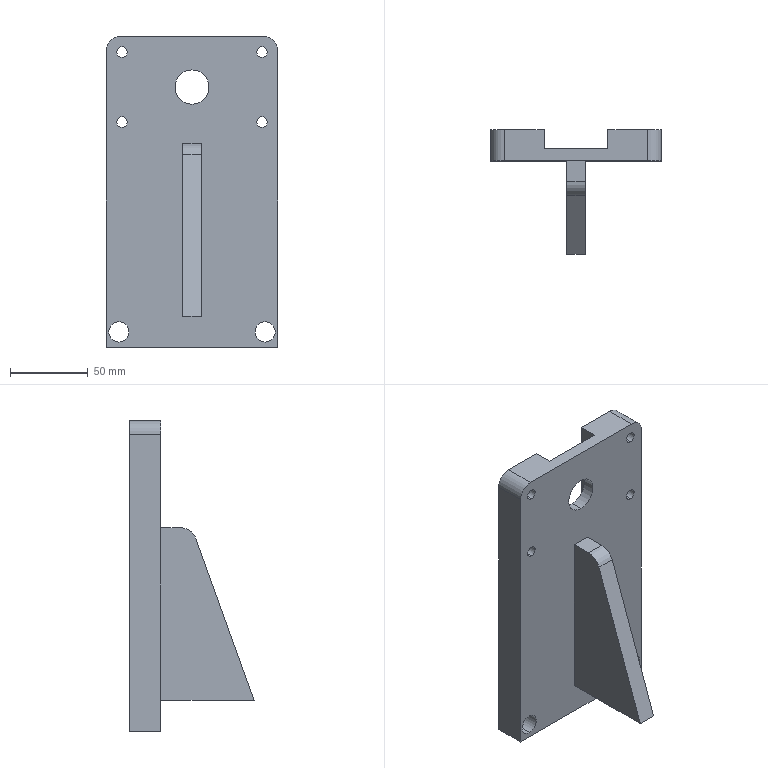Part | SolidWorks | features BaseBody 1 | 1 solid | 32 faces | box 110 x 80 x 200 mm | volume 382814 mm3 | cylinder 17 | plane 15 | commonest cylinder face diameters 6.8 x8 13 x4 18 x2 22 x2 20 x1
STEP:
#1=CARTESIAN_POINT('',(-272.,130.,-29.379));
#2=VERTEX_POINT('',#1);
#3=CARTESIAN_POINT('',(-272.,130.,-16.379));
#4=VERTEX_POINT('',#3);
#5=CARTESIAN_POINT('',(-272.,130.,-22.879));
#6=DIRECTION('',(0.,1.,0.));
#7=DIRECTION('',(0.,0.,1.));
#8=AXIS2_PLACEMENT_3D('',#5,#6,#7);
#9=CIRCLE('',#8,6.5);
#10=EDGE_CURVE('',#2,#4,#9,.T.);
#11=ORIENTED_EDGE('',*,*,#10,.F.);
#12=CARTESIAN_POINT('',(-272.,150.,-29.379));
#13=VERTEX_POINT('',#12);
#14=CARTESIAN_POINT('',(-272.,130.,-29.379));
#15=DIRECTION('',(0.,1.,0.));
#16=VECTOR('',#15,1000.);
#17=LINE('',#14,#16);
#18=EDGE_CURVE('',#2,#13,#17,.T.);
#19=ORIENTED_EDGE('',*,*,#18,.T.);
#20=CARTESIAN_POINT('',(-272.,150.,-16.379));
#21=VERTEX_POINT('',#20);
#22=CARTESIAN_POINT('',(-272.,150.,-22.879));
#23=DIRECTION('',(0.,-1.,0.));
#24=DIRECTION('',(0.,0.,1.));
#25=AXIS2_PLACEMENT_3D('',#22,#23,#24);
#26=CIRCLE('',#25,6.5);
#27=EDGE_CURVE('',#21,#13,#26,.T.);
#28=ORIENTED_EDGE('',*,*,#27,.F.);
#29=CARTESIAN_POINT('',(-272.,130.,-16.379));
#30=DIRECTION('',(0.,1.,0.));
#31=VECTOR('',#30,1000.);
#32=LINE('',#29,#31);
#33=EDGE_CURVE('',#4,#21,#32,.T.);
#34=ORIENTED_EDGE('',*,*,#33,.F.);
#35=EDGE_LOOP('',(#11,#19,#28,#34));
#36=FACE_OUTER_BOUND('',#35,.T.);
#37=CARTESIAN_POINT('',(-272.,130.,-22.879));
#38=DIRECTION('',(0.,1.,0.));
#39=DIRECTION('',(0.,0.,1.));
#40=AXIS2_PLACEMENT_3D('',#37,#38,#39);
#41=CYLINDRICAL_SURFACE('',#40,6.5);
#42=ADVANCED_FACE('',(#36),#41,.F.);
#43=CARTESIAN_POINT('',(-178.,130.,-29.379));
#44=VERTEX_POINT('',#43);
#45=CARTESIAN_POINT('',(-178.,130.,-16.379));
#46=VERTEX_POINT('',#45);
#47=CARTESIAN_POINT('',(-178.,130.,-22.879));
#48=DIRECTION('',(0.,1.,0.));
#49=DIRECTION('',(0.,0.,1.));
#50=AXIS2_PLACEMENT_3D('',#47,#48,#49);
#51=CIRCLE('',#50,6.5);
#52=EDGE_CURVE('',#44,#46,#51,.T.);
#53=ORIENTED_EDGE('',*,*,#52,.F.);
#54=CARTESIAN_POINT('',(-178.,150.,-29.379));
#55=VERTEX_POINT('',#54);
#56=CARTESIAN_POINT('',(-178.,130.,-29.379));
#57=DIRECTION('',(0.,1.,0.));
#58=VECTOR('',#57,1000.);
#59=LINE('',#56,#58);
#60=EDGE_CURVE('',#44,#55,#59,.T.);
#61=ORIENTED_EDGE('',*,*,#60,.T.);
#62=CARTESIAN_POINT('',(-178.,150.,-16.379));
#63=VERTEX_POINT('',#62);
#64=CARTESIAN_POINT('',(-178.,150.,-22.879));
#65=DIRECTION('',(0.,-1.,0.));
#66=DIRECTION('',(0.,0.,1.));
#67=AXIS2_PLACEMENT_3D('',#64,#65,#66);
#68=CIRCLE('',#67,6.5);
#69=EDGE_CURVE('',#63,#55,#68,.T.);
#70=ORIENTED_EDGE('',*,*,#69,.F.);
#71=CARTESIAN_POINT('',(-178.,130.,-16.379));
#72=DIRECTION('',(0.,1.,0.));
#73=VECTOR('',#72,1000.);
#74=LINE('',#71,#73);
#75=EDGE_CURVE('',#46,#63,#74,.T.);
#76=ORIENTED_EDGE('',*,*,#75,.F.);
#77=EDGE_LOOP('',(#53,#61,#70,#76));
#78=FACE_OUTER_BOUND('',#77,.T.);
#79=CARTESIAN_POINT('',(-178.,130.,-22.879));
#80=DIRECTION('',(0.,1.,0.));
#81=DIRECTION('',(0.,0.,1.));
#82=AXIS2_PLACEMENT_3D('',#79,#80,#81);
#83=CYLINDRICAL_SURFACE('',#82,6.5);
#84=ADVANCED_FACE('',(#78),#83,.F.);
#85=CARTESIAN_POINT('',(-180.,130.,108.721));
#86=VERTEX_POINT('',#85);
#87=CARTESIAN_POINT('',(-180.,130.,115.521));
#88=VERTEX_POINT('',#87);
#89=CARTESIAN_POINT('',(-180.,130.,112.121));
#90=DIRECTION('',(0.,1.,0.));
#91=DIRECTION('',(0.,0.,1.));
#92=AXIS2_PLACEMENT_3D('',#89,#90,#91);
#93=CIRCLE('',#92,3.4);
#94=EDGE_CURVE('',#86,#88,#93,.T.);
#95=ORIENTED_EDGE('',*,*,#94,.F.);
#96=CARTESIAN_POINT('',(-180.,150.,108.721));
#97=VERTEX_POINT('',#96);
#98=CARTESIAN_POINT('',(-180.,150.,108.721));
#99=DIRECTION('',(0.,1.,0.));
#100=VECTOR('',#99,1000.);
#101=LINE('',#98,#100);
#102=EDGE_CURVE('',#86,#97,#101,.T.);
#103=ORIENTED_EDGE('',*,*,#102,.T.);
#104=CARTESIAN_POINT('',(-180.,150.,115.521));
#105=VERTEX_POINT('',#104);
#106=CARTESIAN_POINT('',(-180.,150.,112.121));
#107=DIRECTION('',(0.,-1.,0.));
#108=DIRECTION('',(0.,0.,1.));
#109=AXIS2_PLACEMENT_3D('',#106,#107,#108);
#110=CIRCLE('',#109,3.4);
#111=EDGE_CURVE('',#105,#97,#110,.T.);
#112=ORIENTED_EDGE('',*,*,#111,.F.);
#113=CARTESIAN_POINT('',(-180.,150.,115.521));
#114=DIRECTION('',(0.,1.,0.));
#115=VECTOR('',#114,1000.);
#116=LINE('',#113,#115);
#117=EDGE_CURVE('',#88,#105,#116,.T.);
#118=ORIENTED_EDGE('',*,*,#117,.F.);
#119=EDGE_LOOP('',(#95,#103,#112,#118));
#120=FACE_OUTER_BOUND('',#119,.T.);
#121=CARTESIAN_POINT('',(-180.,150.,112.121));
#122=DIRECTION('',(0.,1.,0.));
#123=DIRECTION('',(0.,0.,1.));
#124=AXIS2_PLACEMENT_3D('',#121,#122,#123);
#125=CYLINDRICAL_SURFACE('',#124,3.4);
#126=ADVANCED_FACE('',(#120),#125,.F.);
#127=CARTESIAN_POINT('',(-180.,130.,153.721));
#128=VERTEX_POINT('',#127);
#129=CARTESIAN_POINT('',(-180.,130.,160.521));
#130=VERTEX_POINT('',#129);
#131=CARTESIAN_POINT('',(-180.,130.,157.121));
#132=DIRECTION('',(0.,1.,0.));
#133=DIRECTION('',(0.,0.,1.));
#134=AXIS2_PLACEMENT_3D('',#131,#132,#133);
#135=CIRCLE('',#134,3.4);
#136=EDGE_CURVE('',#128,#130,#135,.T.);
#137=ORIENTED_EDGE('',*,*,#136,.F.);
#138=CARTESIAN_POINT('',(-180.,150.,153.721));
#139=VERTEX_POINT('',#138);
#140=CARTESIAN_POINT('',(-180.,150.,153.721));
#141=DIRECTION('',(0.,1.,0.));
#142=VECTOR('',#141,1000.);
#143=LINE('',#140,#142);
#144=EDGE_CURVE('',#128,#139,#143,.T.);
#145=ORIENTED_EDGE('',*,*,#144,.T.);
#146=CARTESIAN_POINT('',(-180.,150.,160.521));
#147=VERTEX_POINT('',#146);
#148=CARTESIAN_POINT('',(-180.,150.,157.121));
#149=DIRECTION('',(0.,-1.,0.));
#150=DIRECTION('',(0.,0.,1.));
#151=AXIS2_PLACEMENT_3D('',#148,#149,#150);
#152=CIRCLE('',#151,3.4);
#153=EDGE_CURVE('',#147,#139,#152,.T.);
#154=ORIENTED_EDGE('',*,*,#153,.F.);
#155=CARTESIAN_POINT('',(-180.,150.,160.521));
#156=DIRECTION('',(0.,1.,0.));
#157=VECTOR('',#156,1000.);
#158=LINE('',#155,#157);
#159=EDGE_CURVE('',#130,#147,#158,.T.);
#160=ORIENTED_EDGE('',*,*,#159,.F.);
#161=EDGE_LOOP('',(#137,#145,#154,#160));
#162=FACE_OUTER_BOUND('',#161,.T.);
#163=CARTESIAN_POINT('',(-180.,150.,157.121));
#164=DIRECTION('',(0.,1.,0.));
#165=DIRECTION('',(0.,0.,1.));
#166=AXIS2_PLACEMENT_3D('',#163,#164,#165);
#167=CYLINDRICAL_SURFACE('',#166,3.4);
#168=ADVANCED_FACE('',(#162),#167,.F.);
#169=CARTESIAN_POINT('',(-270.,130.,108.721));
#170=VERTEX_POINT('',#169);
#171=CARTESIAN_POINT('',(-270.,130.,115.521));
#172=VERTEX_POINT('',#171);
#173=CARTESIAN_POINT('',(-270.,130.,112.121));
#174=DIRECTION('',(0.,1.,0.));
#175=DIRECTION('',(0.,0.,1.));
#176=AXIS2_PLACEMENT_3D('',#173,#174,#175);
#177=CIRCLE('',#176,3.4);
#178=EDGE_CURVE('',#170,#172,#177,.T.);
#179=ORIENTED_EDGE('',*,*,#178,.F.);
#180=CARTESIAN_POINT('',(-270.,150.,108.721));
#181=VERTEX_POINT('',#180);
#182=CARTESIAN_POINT('',(-270.,150.,108.721));
#183=DIRECTION('',(0.,1.,0.));
#184=VECTOR('',#183,1000.);
#185=LINE('',#182,#184);
#186=EDGE_CURVE('',#170,#181,#185,.T.);
#187=ORIENTED_EDGE('',*,*,#186,.T.);
#188=CARTESIAN_POINT('',(-270.,150.,115.521));
#189=VERTEX_POINT('',#188);
#190=CARTESIAN_POINT('',(-270.,150.,112.121));
#191=DIRECTION('',(0.,-1.,0.));
#192=DIRECTION('',(0.,0.,1.));
#193=AXIS2_PLACEMENT_3D('',#190,#191,#192);
#194=CIRCLE('',#193,3.4);
#195=EDGE_CURVE('',#189,#181,#194,.T.);
#196=ORIENTED_EDGE('',*,*,#195,.F.);
#197=CARTESIAN_POINT('',(-270.,150.,115.521));
#198=DIRECTION('',(0.,1.,0.));
#199=VECTOR('',#198,1000.);
#200=LINE('',#197,#199);
#201=EDGE_CURVE('',#172,#189,#200,.T.);
#202=ORIENTED_EDGE('',*,*,#201,.F.);
#203=EDGE_LOOP('',(#179,#187,#196,#202));
#204=FACE_OUTER_BOUND('',#203,.T.);
#205=CARTESIAN_POINT('',(-270.,150.,112.121));
#206=DIRECTION('',(0.,1.,0.));
#207=DIRECTION('',(0.,0.,1.));
#208=AXIS2_PLACEMENT_3D('',#205,#206,#207);
#209=CYLINDRICAL_SURFACE('',#208,3.4);
#210=ADVANCED_FACE('',(#204),#209,.F.);
#211=CARTESIAN_POINT('',(-270.,130.,153.721));
#212=VERTEX_POINT('',#211);
#213=CARTESIAN_POINT('',(-270.,130.,160.521));
#214=VERTEX_POINT('',#213);
#215=CARTESIAN_POINT('',(-270.,130.,157.121));
#216=DIRECTION('',(0.,1.,0.));
#217=DIRECTION('',(0.,0.,1.));
#218=AXIS2_PLACEMENT_3D('',#215,#216,#217);
#219=CIRCLE('',#218,3.4);
#220=EDGE_CURVE('',#212,#214,#219,.T.);
#221=ORIENTED_EDGE('',*,*,#220,.F.);
#222=CARTESIAN_POINT('',(-270.,150.,153.721));
#223=VERTEX_POINT('',#222);
#224=CARTESIAN_POINT('',(-270.,150.,153.721));
#225=DIRECTION('',(0.,1.,0.));
#226=VECTOR('',#225,1000.);
#227=LINE('',#224,#226);
#228=EDGE_CURVE('',#212,#223,#227,.T.);
#229=ORIENTED_EDGE('',*,*,#228,.T.);
#230=CARTESIAN_POINT('',(-270.,150.,160.521));
#231=VERTEX_POINT('',#230);
#232=CARTESIAN_POINT('',(-270.,150.,157.121));
#233=DIRECTION('',(0.,-1.,0.));
#234=DIRECTION('',(0.,0.,1.));
#235=AXIS2_PLACEMENT_3D('',#232,#233,#234);
#236=CIRCLE('',#235,3.4);
#237=EDGE_CURVE('',#231,#223,#236,.T.);
#238=ORIENTED_EDGE('',*,*,#237,.F.);
#239=CARTESIAN_POINT('',(-270.,150.,160.521));
#240=DIRECTION('',(0.,1.,0.));
#241=VECTOR('',#240,1000.);
#242=LINE('',#239,#241);
#243=EDGE_CURVE('',#214,#231,#242,.T.);
#244=ORIENTED_EDGE('',*,*,#243,.F.);
#245=EDGE_LOOP('',(#221,#229,#238,#244));
#246=FACE_OUTER_BOUND('',#245,.T.);
#247=CARTESIAN_POINT('',(-270.,150.,157.121));
#248=DIRECTION('',(0.,1.,0.));
#249=DIRECTION('',(0.,0.,1.));
#250=AXIS2_PLACEMENT_3D('',#247,#248,#249);
#251=CYLINDRICAL_SURFACE('',#250,3.4);
#252=ADVANCED_FACE('',(#246),#251,.F.);
#253=CARTESIAN_POINT('',(-225.,130.,123.621));
#254=VERTEX_POINT('',#253);
#255=CARTESIAN_POINT('',(-225.,130.,145.621));
#256=VERTEX_POINT('',#255);
#257=CARTESIAN_POINT('',(-225.,130.,134.621));
#258=DIRECTION('',(0.,1.,0.));
#259=DIRECTION('',(0.,0.,1.));
#260=AXIS2_PLACEMENT_3D('',#257,#258,#259);
#261=CIRCLE('',#260,11.);
#262=EDGE_CURVE('',#254,#256,#261,.T.);
#263=ORIENTED_EDGE('',*,*,#262,.F.);
#264=CARTESIAN_POINT('',(-225.,138.,123.621));
#265=VERTEX_POINT('',#264);
#266=CARTESIAN_POINT('',(-225.,129.999,123.621));
#267=DIRECTION('',(0.,1.,0.));
#268=VECTOR('',#267,1000.);
#269=LINE('',#266,#268);
#270=EDGE_CURVE('',#254,#265,#269,.T.);
#271=ORIENTED_EDGE('',*,*,#270,.T.);
#272=CARTESIAN_POINT('',(-225.,138.,145.621));
#273=VERTEX_POINT('',#272);
#274=CARTESIAN_POINT('',(-225.,138.,134.621));
#275=DIRECTION('',(0.,-1.,0.));
#276=DIRECTION('',(0.,0.,1.));
#277=AXIS2_PLACEMENT_3D('',#274,#275,#276);
#278=CIRCLE('',#277,11.);
#279=EDGE_CURVE('',#273,#265,#278,.T.);
#280=ORIENTED_EDGE('',*,*,#279,.F.);
#281=CARTESIAN_POINT('',(-225.,129.999,145.621));
#282=DIRECTION('',(0.,1.,0.));
#283=VECTOR('',#282,1000.);
#284=LINE('',#281,#283);
#285=EDGE_CURVE('',#256,#273,#284,.T.);
#286=ORIENTED_EDGE('',*,*,#285,.F.);
#287=EDGE_LOOP('',(#263,#271,#280,#286));
#288=FACE_OUTER_BOUND('',#287,.T.);
#289=CARTESIAN_POINT('',(-225.,129.999,134.621));
#290=DIRECTION('',(0.,1.,0.));
#291=DIRECTION('',(0.,0.,1.));
#292=AXIS2_PLACEMENT_3D('',#289,#290,#291);
#293=CYLINDRICAL_SURFACE('',#292,11.);
#294=ADVANCED_FACE('',(#288),#293,.F.);
#295=CARTESIAN_POINT('',(-219.,130.,-12.879));
#296=VERTEX_POINT('',#295);
#297=CARTESIAN_POINT('',(-231.,130.,-12.879));
#298=VERTEX_POINT('',#297);
#299=CARTESIAN_POINT('',(-225.,130.,-12.879));
#300=DIRECTION('',(-1.,0.,0.));
#301=VECTOR('',#300,1000.);
#302=LINE('',#299,#301);
#303=EDGE_CURVE('',#296,#298,#302,.T.);
#304=ORIENTED_EDGE('',*,*,#303,.T.);
#305=CARTESIAN_POINT('',(-231.,130.,98.107));
#306=VERTEX_POINT('',#305);
#307=CARTESIAN_POINT('',(-231.,130.,67.121));
#308=DIRECTION('',(0.,0.,1.));
#309=VECTOR('',#308,1000.);
#310=LINE('',#307,#309);
#311=EDGE_CURVE('',#298,#306,#310,.T.);
#312=ORIENTED_EDGE('',*,*,#311,.T.);
#313=CARTESIAN_POINT('',(-219.,130.,98.107));
#314=VERTEX_POINT('',#313);
#315=CARTESIAN_POINT('',(-225.,130.,98.107));
#316=DIRECTION('',(1.,0.,0.));
#317=VECTOR('',#316,1000.);
#318=LINE('',#315,#317);
#319=EDGE_CURVE('',#306,#314,#318,.T.);
#320=ORIENTED_EDGE('',*,*,#319,.T.);
#321=CARTESIAN_POINT('',(-219.,130.,67.121));
#322=DIRECTION('',(0.,0.,-1.));
#323=VECTOR('',#322,1000.);
#324=LINE('',#321,#323);
#325=EDGE_CURVE('',#314,#296,#324,.T.);
#326=ORIENTED_EDGE('',*,*,#325,.T.);
#327=EDGE_LOOP('',(#304,#312,#320,#326));
#328=FACE_BOUND('',#327,.T.);
#329=CARTESIAN_POINT('',(-272.,130.,-22.879));
#330=DIRECTION('',(0.,1.,0.));
#331=DIRECTION('',(0.,0.,1.));
#332=AXIS2_PLACEMENT_3D('',#329,#330,#331);
#333=CIRCLE('',#332,6.5);
#334=EDGE_CURVE('',#4,#2,#333,.T.);
#335=ORIENTED_EDGE('',*,*,#334,.T.);
#336=ORIENTED_EDGE('',*,*,#10,.T.);
#337=EDGE_LOOP('',(#335,#336));
#338=FACE_BOUND('',#337,.T.);
#339=CARTESIAN_POINT('',(-178.,130.,-22.879));
#340=DIRECTION('',(0.,1.,0.));
#341=DIRECTION('',(0.,0.,1.));
#342=AXIS2_PLACEMENT_3D('',#339,#340,#341);
#343=CIRCLE('',#342,6.5);
#344=EDGE_CURVE('',#46,#44,#343,.T.);
#345=ORIENTED_EDGE('',*,*,#344,.T.);
#346=ORIENTED_EDGE('',*,*,#52,.T.);
#347=EDGE_LOOP('',(#345,#346));
#348=FACE_BOUND('',#347,.T.);
#349=CARTESIAN_POINT('',(-180.,130.,112.121));
#350=DIRECTION('',(0.,1.,0.));
#351=DIRECTION('',(0.,0.,1.));
#352=AXIS2_PLACEMENT_3D('',#349,#350,#351);
#353=CIRCLE('',#352,3.4);
#354=EDGE_CURVE('',#88,#86,#353,.T.);
#355=ORIENTED_EDGE('',*,*,#354,.T.);
#356=ORIENTED_EDGE('',*,*,#94,.T.);
#357=EDGE_LOOP('',(#355,#356));
#358=FACE_BOUND('',#357,.T.);
#359=CARTESIAN_POINT('',(-180.,130.,157.121));
#360=DIRECTION('',(0.,1.,0.));
#361=DIRECTION('',(0.,0.,1.));
#362=AXIS2_PLACEMENT_3D('',#359,#360,#361);
#363=CIRCLE('',#362,3.4);
#364=EDGE_CURVE('',#130,#128,#363,.T.);
#365=ORIENTED_EDGE('',*,*,#364,.T.);
#366=ORIENTED_EDGE('',*,*,#136,.T.);
#367=EDGE_LOOP('',(#365,#366));
#368=FACE_BOUND('',#367,.T.);
#369=CARTESIAN_POINT('',(-270.,130.,112.121));
#370=DIRECTION('',(0.,1.,0.));
#371=DIRECTION('',(0.,0.,1.));
#372=AXIS2_PLACEMENT_3D('',#369,#370,#371);
#373=CIRCLE('',#372,3.4);
#374=EDGE_CURVE('',#172,#170,#373,.T.);
#375=ORIENTED_EDGE('',*,*,#374,.T.);
#376=ORIENTED_EDGE('',*,*,#178,.T.);
#377=EDGE_LOOP('',(#375,#376));
#378=FACE_BOUND('',#377,.T.);
#379=CARTESIAN_POINT('',(-270.,130.,157.121));
#380=DIRECTION('',(0.,1.,0.));
#381=DIRECTION('',(0.,0.,1.));
#382=AXIS2_PLACEMENT_3D('',#379,#380,#381);
#383=CIRCLE('',#382,3.4);
#384=EDGE_CURVE('',#214,#212,#383,.T.);
#385=ORIENTED_EDGE('',*,*,#384,.T.);
#386=ORIENTED_EDGE('',*,*,#220,.T.);
#387=EDGE_LOOP('',(#385,#386));
#388=FACE_BOUND('',#387,.T.);
#389=CARTESIAN_POINT('',(-225.,130.,134.621));
#390=DIRECTION('',(0.,1.,0.));
#391=DIRECTION('',(0.,0.,1.));
#392=AXIS2_PLACEMENT_3D('',#389,#390,#391);
#393=CIRCLE('',#392,11.);
#394=EDGE_CURVE('',#256,#254,#393,.T.);
#395=ORIENTED_EDGE('',*,*,#394,.T.);
#396=ORIENTED_EDGE('',*,*,#262,.T.);
#397=EDGE_LOOP('',(#395,#396));
#398=FACE_BOUND('',#397,.T.);
#399=CARTESIAN_POINT('',(-280.,130.,158.121));
#400=VERTEX_POINT('',#399);
#401=CARTESIAN_POINT('',(-280.,130.,-32.879));
#402=VERTEX_POINT('',#401);
#403=CARTESIAN_POINT('',(-280.,130.,67.121));
#404=DIRECTION('',(0.,0.,-1.));
#405=VECTOR('',#404,1000.);
#406=LINE('',#403,#405);
#407=EDGE_CURVE('',#400,#402,#406,.T.);
#408=ORIENTED_EDGE('',*,*,#407,.T.);
#409=CARTESIAN_POINT('',(-170.,130.,-32.879));
#410=VERTEX_POINT('',#409);
#411=CARTESIAN_POINT('',(-225.,130.,-32.879));
#412=DIRECTION('',(1.,0.,0.));
#413=VECTOR('',#412,1000.);
#414=LINE('',#411,#413);
#415=EDGE_CURVE('',#402,#410,#414,.T.);
#416=ORIENTED_EDGE('',*,*,#415,.T.);
#417=CARTESIAN_POINT('',(-170.,130.,158.121));
#418=VERTEX_POINT('',#417);
#419=CARTESIAN_POINT('',(-170.,130.,67.121));
#420=DIRECTION('',(0.,0.,1.));
#421=VECTOR('',#420,1000.);
#422=LINE('',#419,#421);
#423=EDGE_CURVE('',#410,#418,#422,.T.);
#424=ORIENTED_EDGE('',*,*,#423,.T.);
#425=CARTESIAN_POINT('',(-179.,130.,167.121));
#426=VERTEX_POINT('',#425);
#427=CARTESIAN_POINT('',(-179.,130.,158.121));
#428=DIRECTION('',(0.,-1.,0.));
#429=DIRECTION('',(0.,0.,-1.));
#430=AXIS2_PLACEMENT_3D('',#427,#428,#429);
#431=CIRCLE('',#430,9.);
#432=EDGE_CURVE('',#418,#426,#431,.T.);
#433=ORIENTED_EDGE('',*,*,#432,.T.);
#434=CARTESIAN_POINT('',(-271.,130.,167.121));
#435=VERTEX_POINT('',#434);
#436=CARTESIAN_POINT('',(-225.,130.,167.121));
#437=DIRECTION('',(-1.,0.,0.));
#438=VECTOR('',#437,1000.);
#439=LINE('',#436,#438);
#440=EDGE_CURVE('',#426,#435,#439,.T.);
#441=ORIENTED_EDGE('',*,*,#440,.T.);
#442=CARTESIAN_POINT('',(-271.,130.,158.121));
#443=DIRECTION('',(0.,-1.,0.));
#444=DIRECTION('',(0.,0.,-1.));
#445=AXIS2_PLACEMENT_3D('',#442,#443,#444);
#446=CIRCLE('',#445,9.);
#447=EDGE_CURVE('',#435,#400,#446,.T.);
#448=ORIENTED_EDGE('',*,*,#447,.T.);
#449=EDGE_LOOP('',(#408,#416,#424,#433,#441,#448));
#450=FACE_OUTER_BOUND('',#449,.T.);
#451=CARTESIAN_POINT('',(-225.,130.,67.121));
#452=DIRECTION('',(0.,-1.,0.));
#453=DIRECTION('',(0.,0.,-1.));
#454=AXIS2_PLACEMENT_3D('',#451,#452,#453);
#455=PLANE('',#454);
#456=ADVANCED_FACE('',(#328,#338,#348,#358,#368,#378,#388,#398,#450),#455,.T.);
#457=ORIENTED_EDGE('',*,*,#311,.F.);
#458=CARTESIAN_POINT('',(-231.,70.,-12.879));
#459=VERTEX_POINT('',#458);
#460=CARTESIAN_POINT('',(-231.,130.,-12.879));
#461=DIRECTION('',(0.,-1.,0.));
#462=VECTOR('',#461,1000.);
#463=LINE('',#460,#462);
#464=EDGE_CURVE('',#298,#459,#463,.T.);
#465=ORIENTED_EDGE('',*,*,#464,.T.);
#466=CARTESIAN_POINT('',(-231.,107.618,91.497));
#467=VERTEX_POINT('',#466);
#468=CARTESIAN_POINT('',(-231.,70.,-12.879));
#469=DIRECTION('',(0.,0.3391,0.9408));
#470=VECTOR('',#469,1000.);
#471=LINE('',#468,#470);
#472=EDGE_CURVE('',#459,#467,#471,.T.);
#473=ORIENTED_EDGE('',*,*,#472,.T.);
#474=CARTESIAN_POINT('',(-231.,117.026,98.107));
#475=VERTEX_POINT('',#474);
#476=CARTESIAN_POINT('',(-231.,117.026,88.107));
#477=DIRECTION('',(-1.,0.,0.));
#478=DIRECTION('',(0.,0.,1.));
#479=AXIS2_PLACEMENT_3D('',#476,#477,#478);
#480=CIRCLE('',#479,10.);
#481=EDGE_CURVE('',#467,#475,#480,.T.);
#482=ORIENTED_EDGE('',*,*,#481,.T.);
#483=CARTESIAN_POINT('',(-231.,130.,98.107));
#484=DIRECTION('',(0.,1.,0.));
#485=VECTOR('',#484,1000.);
#486=LINE('',#483,#485);
#487=EDGE_CURVE('',#475,#306,#486,.T.);
#488=ORIENTED_EDGE('',*,*,#487,.T.);
#489=EDGE_LOOP('',(#457,#465,#473,#482,#488));
#490=FACE_OUTER_BOUND('',#489,.T.);
#491=CARTESIAN_POINT('',(-231.,130.,67.121));
#492=DIRECTION('',(-1.,0.,0.));
#493=DIRECTION('',(0.,0.,1.));
#494=AXIS2_PLACEMENT_3D('',#491,#492,#493);
#495=PLANE('',#494);
#496=ADVANCED_FACE('',(#490),#495,.T.);
#497=ORIENTED_EDGE('',*,*,#303,.F.);
#498=CARTESIAN_POINT('',(-219.,70.,-12.879));
#499=VERTEX_POINT('',#498);
#500=CARTESIAN_POINT('',(-219.,130.,-12.879));
#501=DIRECTION('',(0.,1.,0.));
#502=VECTOR('',#501,1000.);
#503=LINE('',#500,#502);
#504=EDGE_CURVE('',#499,#296,#503,.T.);
#505=ORIENTED_EDGE('',*,*,#504,.F.);
#506=CARTESIAN_POINT('',(-219.,70.,-12.879));
#507=DIRECTION('',(1.,0.,0.));
#508=VECTOR('',#507,1000.);
#509=LINE('',#506,#508);
#510=EDGE_CURVE('',#459,#499,#509,.T.);
#511=ORIENTED_EDGE('',*,*,#510,.F.);
#512=ORIENTED_EDGE('',*,*,#464,.F.);
#513=EDGE_LOOP('',(#497,#505,#511,#512));
#514=FACE_OUTER_BOUND('',#513,.T.);
#515=CARTESIAN_POINT('',(-219.,130.,-12.879));
#516=DIRECTION('',(0.,0.,1.));
#517=DIRECTION('',(1.,0.,0.));
#518=AXIS2_PLACEMENT_3D('',#515,#516,#517);
#519=PLANE('',#518);
#520=ADVANCED_FACE('',(#514),#519,.F.);
#521=CARTESIAN_POINT('',(-219.,107.618,91.497));
#522=VERTEX_POINT('',#521);
#523=CARTESIAN_POINT('',(-219.,117.026,98.107));
#524=VERTEX_POINT('',#523);
#525=CARTESIAN_POINT('',(-219.,117.026,88.107));
#526=DIRECTION('',(-1.,0.,0.));
#527=DIRECTION('',(0.,0.,1.));
#528=AXIS2_PLACEMENT_3D('',#525,#526,#527);
#529=CIRCLE('',#528,10.);
#530=EDGE_CURVE('',#522,#524,#529,.T.);
#531=ORIENTED_EDGE('',*,*,#530,.F.);
#532=CARTESIAN_POINT('',(-219.,70.,-12.879));
#533=DIRECTION('',(0.,0.3391,0.9408));
#534=VECTOR('',#533,1000.);
#535=LINE('',#532,#534);
#536=EDGE_CURVE('',#499,#522,#535,.T.);
#537=ORIENTED_EDGE('',*,*,#536,.F.);
#538=ORIENTED_EDGE('',*,*,#504,.T.);
#539=ORIENTED_EDGE('',*,*,#325,.F.);
#540=CARTESIAN_POINT('',(-219.,130.,98.107));
#541=DIRECTION('',(0.,1.,0.));
#542=VECTOR('',#541,1000.);
#543=LINE('',#540,#542);
#544=EDGE_CURVE('',#524,#314,#543,.T.);
#545=ORIENTED_EDGE('',*,*,#544,.F.);
#546=EDGE_LOOP('',(#531,#537,#538,#539,#545));
#547=FACE_OUTER_BOUND('',#546,.T.);
#548=CARTESIAN_POINT('',(-219.,130.,67.121));
#549=DIRECTION('',(-1.,0.,0.));
#550=DIRECTION('',(0.,0.,1.));
#551=AXIS2_PLACEMENT_3D('',#548,#549,#550);
#552=PLANE('',#551);
#553=ADVANCED_FACE('',(#547),#552,.F.);
#554=CARTESIAN_POINT('',(-219.,117.026,98.107));
#555=DIRECTION('',(-1.,0.,0.));
#556=VECTOR('',#555,1000.);
#557=LINE('',#554,#556);
#558=EDGE_CURVE('',#524,#475,#557,.T.);
#559=ORIENTED_EDGE('',*,*,#558,.F.);
#560=ORIENTED_EDGE('',*,*,#544,.T.);
#561=ORIENTED_EDGE('',*,*,#319,.F.);
#562=ORIENTED_EDGE('',*,*,#487,.F.);
#563=EDGE_LOOP('',(#559,#560,#561,#562));
#564=FACE_OUTER_BOUND('',#563,.T.);
#565=CARTESIAN_POINT('',(-219.,130.,98.107));
#566=DIRECTION('',(0.,0.,-1.));
#567=DIRECTION('',(-1.,0.,0.));
#568=AXIS2_PLACEMENT_3D('',#565,#566,#567);
#569=PLANE('',#568);
#570=ADVANCED_FACE('',(#564),#569,.F.);
#571=ORIENTED_EDGE('',*,*,#18,.F.);
#572=ORIENTED_EDGE('',*,*,#334,.F.);
#573=ORIENTED_EDGE('',*,*,#33,.T.);
#574=CARTESIAN_POINT('',(-272.,150.,-22.879));
#575=DIRECTION('',(0.,-1.,0.));
#576=DIRECTION('',(0.,0.,1.));
#577=AXIS2_PLACEMENT_3D('',#574,#575,#576);
#578=CIRCLE('',#577,6.5);
#579=EDGE_CURVE('',#13,#21,#578,.T.);
#580=ORIENTED_EDGE('',*,*,#579,.F.);
#581=EDGE_LOOP('',(#571,#572,#573,#580));
#582=FACE_OUTER_BOUND('',#581,.T.);
#583=CARTESIAN_POINT('',(-272.,130.,-22.879));
#584=DIRECTION('',(0.,1.,0.));
#585=DIRECTION('',(0.,0.,1.));
#586=AXIS2_PLACEMENT_3D('',#583,#584,#585);
#587=CYLINDRICAL_SURFACE('',#586,6.5);
#588=ADVANCED_FACE('',(#582),#587,.F.);
#589=ORIENTED_EDGE('',*,*,#60,.F.);
#590=ORIENTED_EDGE('',*,*,#344,.F.);
#591=ORIENTED_EDGE('',*,*,#75,.T.);
#592=CARTESIAN_POINT('',(-178.,150.,-22.879));
#593=DIRECTION('',(0.,-1.,0.));
#594=DIRECTION('',(0.,0.,1.));
#595=AXIS2_PLACEMENT_3D('',#592,#593,#594);
#596=CIRCLE('',#595,6.5);
#597=EDGE_CURVE('',#55,#63,#596,.T.);
#598=ORIENTED_EDGE('',*,*,#597,.F.);
#599=EDGE_LOOP('',(#589,#590,#591,#598));
#600=FACE_OUTER_BOUND('',#599,.T.);
#601=CARTESIAN_POINT('',(-178.,130.,-22.879));
#602=DIRECTION('',(0.,1.,0.));
#603=DIRECTION('',(0.,0.,1.));
#604=AXIS2_PLACEMENT_3D('',#601,#602,#603);
#605=CYLINDRICAL_SURFACE('',#604,6.5);
#606=ADVANCED_FACE('',(#600),#605,.F.);
#607=ORIENTED_EDGE('',*,*,#102,.F.);
#608=ORIENTED_EDGE('',*,*,#354,.F.);
#609=ORIENTED_EDGE('',*,*,#117,.T.);
#610=CARTESIAN_POINT('',(-180.,150.,112.121));
#611=DIRECTION('',(0.,-1.,0.));
#612=DIRECTION('',(0.,0.,1.));
#613=AXIS2_PLACEMENT_3D('',#610,#611,#612);
#614=CIRCLE('',#613,3.4);
#615=EDGE_CURVE('',#97,#105,#614,.T.);
#616=ORIENTED_EDGE('',*,*,#615,.F.);
#617=EDGE_LOOP('',(#607,#608,#609,#616));
#618=FACE_OUTER_BOUND('',#617,.T.);
#619=CARTESIAN_POINT('',(-180.,150.,112.121));
#620=DIRECTION('',(0.,1.,0.));
#621=DIRECTION('',(0.,0.,1.));
#622=AXIS2_PLACEMENT_3D('',#619,#620,#621);
#623=CYLINDRICAL_SURFACE('',#622,3.4);
#624=ADVANCED_FACE('',(#618),#623,.F.);
#625=ORIENTED_EDGE('',*,*,#144,.F.);
#626=ORIENTED_EDGE('',*,*,#364,.F.);
#627=ORIENTED_EDGE('',*,*,#159,.T.);
#628=CARTESIAN_POINT('',(-180.,150.,157.121));
#629=DIRECTION('',(0.,-1.,0.));
#630=DIRECTION('',(0.,0.,1.));
#631=AXIS2_PLACEMENT_3D('',#628,#629,#630);
#632=CIRCLE('',#631,3.4);
#633=EDGE_CURVE('',#139,#147,#632,.T.);
#634=ORIENTED_EDGE('',*,*,#633,.F.);
#635=EDGE_LOOP('',(#625,#626,#627,#634));
#636=FACE_OUTER_BOUND('',#635,.T.);
#637=CARTESIAN_POINT('',(-180.,150.,157.121));
#638=DIRECTION('',(0.,1.,0.));
#639=DIRECTION('',(0.,0.,1.));
#640=AXIS2_PLACEMENT_3D('',#637,#638,#639);
#641=CYLINDRICAL_SURFACE('',#640,3.4);
#642=ADVANCED_FACE('',(#636),#641,.F.);
#643=ORIENTED_EDGE('',*,*,#186,.F.);
#644=ORIENTED_EDGE('',*,*,#374,.F.);
#645=ORIENTED_EDGE('',*,*,#201,.T.);
#646=CARTESIAN_POINT('',(-270.,150.,112.121));
#647=DIRECTION('',(0.,-1.,0.));
#648=DIRECTION('',(0.,0.,1.));
#649=AXIS2_PLACEMENT_3D('',#646,#647,#648);
#650=CIRCLE('',#649,3.4);
#651=EDGE_CURVE('',#181,#189,#650,.T.);
#652=ORIENTED_EDGE('',*,*,#651,.F.);
#653=EDGE_LOOP('',(#643,#644,#645,#652));
#654=FACE_OUTER_BOUND('',#653,.T.);
#655=CARTESIAN_POINT('',(-270.,150.,112.121));
#656=DIRECTION('',(0.,1.,0.));
#657=DIRECTION('',(0.,0.,1.));
#658=AXIS2_PLACEMENT_3D('',#655,#656,#657);
#659=CYLINDRICAL_SURFACE('',#658,3.4);
#660=ADVANCED_FACE('',(#654),#659,.F.);
#661=ORIENTED_EDGE('',*,*,#228,.F.);
#662=ORIENTED_EDGE('',*,*,#384,.F.);
#663=ORIENTED_EDGE('',*,*,#243,.T.);
#664=CARTESIAN_POINT('',(-270.,150.,157.121));
#665=DIRECTION('',(0.,-1.,0.));
#666=DIRECTION('',(0.,0.,1.));
#667=AXIS2_PLACEMENT_3D('',#664,#665,#666);
#668=CIRCLE('',#667,3.4);
#669=EDGE_CURVE('',#223,#231,#668,.T.);
#670=ORIENTED_EDGE('',*,*,#669,.F.);
#671=EDGE_LOOP('',(#661,#662,#663,#670));
#672=FACE_OUTER_BOUND('',#671,.T.);
#673=CARTESIAN_POINT('',(-270.,150.,157.121));
#674=DIRECTION('',(0.,1.,0.));
#675=DIRECTION('',(0.,0.,1.));
#676=AXIS2_PLACEMENT_3D('',#673,#674,#675);
#677=CYLINDRICAL_SURFACE('',#676,3.4);
#678=ADVANCED_FACE('',(#672),#677,.F.);
#679=ORIENTED_EDGE('',*,*,#270,.F.);
#680=ORIENTED_EDGE('',*,*,#394,.F.);
#681=ORIENTED_EDGE('',*,*,#285,.T.);
#682=CARTESIAN_POINT('',(-225.,138.,134.621));
#683=DIRECTION('',(0.,-1.,0.));
#684=DIRECTION('',(0.,0.,1.));
#685=AXIS2_PLACEMENT_3D('',#682,#683,#684);
#686=CIRCLE('',#685,11.);
#687=EDGE_CURVE('',#265,#273,#686,.T.);
#688=ORIENTED_EDGE('',*,*,#687,.F.);
#689=EDGE_LOOP('',(#679,#680,#681,#688));
#690=FACE_OUTER_BOUND('',#689,.T.);
#691=CARTESIAN_POINT('',(-225.,129.999,134.621));
#692=DIRECTION('',(0.,1.,0.));
#693=DIRECTION('',(0.,0.,1.));
#694=AXIS2_PLACEMENT_3D('',#691,#692,#693);
#695=CYLINDRICAL_SURFACE('',#694,11.);
#696=ADVANCED_FACE('',(#690),#695,.F.);
#697=CARTESIAN_POINT('',(-204.5,150.,-32.879));
#698=VERTEX_POINT('',#697);
#699=CARTESIAN_POINT('',(-204.5,138.,-32.879));
#700=VERTEX_POINT('',#699);
#701=CARTESIAN_POINT('',(-204.5,150.,-32.879));
#702=DIRECTION('',(0.,-1.,0.));
#703=VECTOR('',#702,1000.);
#704=LINE('',#701,#703);
#705=EDGE_CURVE('',#698,#700,#704,.T.);
#706=ORIENTED_EDGE('',*,*,#705,.F.);
#707=CARTESIAN_POINT('',(-170.,150.,-32.879));
#708=VERTEX_POINT('',#707);
#709=CARTESIAN_POINT('',(-280.,150.,-32.879));
#710=DIRECTION('',(-1.,0.,0.));
#711=VECTOR('',#710,1000.);
#712=LINE('',#709,#711);
#713=EDGE_CURVE('',#708,#698,#712,.T.);
#714=ORIENTED_EDGE('',*,*,#713,.F.);
#715=CARTESIAN_POINT('',(-170.,150.,-32.879));
#716=DIRECTION('',(0.,1.,0.));
#717=VECTOR('',#716,1000.);
#718=LINE('',#715,#717);
#719=EDGE_CURVE('',#410,#708,#718,.T.);
#720=ORIENTED_EDGE('',*,*,#719,.F.);
#721=ORIENTED_EDGE('',*,*,#415,.F.);
#722=CARTESIAN_POINT('',(-280.,150.,-32.879));
#723=VERTEX_POINT('',#722);
#724=CARTESIAN_POINT('',(-280.,150.,-32.879));
#725=DIRECTION('',(0.,-1.,0.));
#726=VECTOR('',#725,1000.);
#727=LINE('',#724,#726);
#728=EDGE_CURVE('',#723,#402,#727,.T.);
#729=ORIENTED_EDGE('',*,*,#728,.F.);
#730=CARTESIAN_POINT('',(-245.5,150.,-32.879));
#731=VERTEX_POINT('',#730);
#732=CARTESIAN_POINT('',(-280.,150.,-32.879));
#733=DIRECTION('',(-1.,0.,0.));
#734=VECTOR('',#733,1000.);
#735=LINE('',#732,#734);
#736=EDGE_CURVE('',#731,#723,#735,.T.);
#737=ORIENTED_EDGE('',*,*,#736,.F.);
#738=CARTESIAN_POINT('',(-245.5,138.,-32.879));
#739=VERTEX_POINT('',#738);
#740=CARTESIAN_POINT('',(-245.5,150.,-32.879));
#741=DIRECTION('',(0.,1.,0.));
#742=VECTOR('',#741,1000.);
#743=LINE('',#740,#742);
#744=EDGE_CURVE('',#739,#731,#743,.T.);
#745=ORIENTED_EDGE('',*,*,#744,.F.);
#746=CARTESIAN_POINT('',(-280.,138.,-32.879));
#747=DIRECTION('',(-1.,0.,0.));
#748=VECTOR('',#747,1000.);
#749=LINE('',#746,#748);
#750=EDGE_CURVE('',#700,#739,#749,.T.);
#751=ORIENTED_EDGE('',*,*,#750,.F.);
#752=EDGE_LOOP('',(#706,#714,#720,#721,#729,#737,#745,#751));
#753=FACE_OUTER_BOUND('',#752,.T.);
#754=CARTESIAN_POINT('',(-280.,150.,-32.879));
#755=DIRECTION('',(0.,0.,1.));
#756=DIRECTION('',(1.,0.,0.));
#757=AXIS2_PLACEMENT_3D('',#754,#755,#756);
#758=PLANE('',#757);
#759=ADVANCED_FACE('',(#753),#758,.F.);
#760=CARTESIAN_POINT('',(-280.,150.,158.121));
#761=VERTEX_POINT('',#760);
#762=CARTESIAN_POINT('',(-280.,150.,158.121));
#763=DIRECTION('',(0.,-1.,0.));
#764=VECTOR('',#763,1000.);
#765=LINE('',#762,#764);
#766=EDGE_CURVE('',#761,#400,#765,.T.);
#767=ORIENTED_EDGE('',*,*,#766,.F.);
#768=CARTESIAN_POINT('',(-280.,150.,167.121));
#769=DIRECTION('',(0.,0.,1.));
#770=VECTOR('',#769,1000.);
#771=LINE('',#768,#770);
#772=EDGE_CURVE('',#723,#761,#771,.T.);
#773=ORIENTED_EDGE('',*,*,#772,.F.);
#774=ORIENTED_EDGE('',*,*,#728,.T.);
#775=ORIENTED_EDGE('',*,*,#407,.F.);
#776=EDGE_LOOP('',(#767,#773,#774,#775));
#777=FACE_OUTER_BOUND('',#776,.T.);
#778=CARTESIAN_POINT('',(-280.,150.,167.121));
#779=DIRECTION('',(1.,0.,0.));
#780=DIRECTION('',(0.,0.,-1.));
#781=AXIS2_PLACEMENT_3D('',#778,#779,#780);
#782=PLANE('',#781);
#783=ADVANCED_FACE('',(#777),#782,.F.);
#784=ORIENTED_EDGE('',*,*,#447,.F.);
#785=CARTESIAN_POINT('',(-271.,150.,167.121));
#786=VERTEX_POINT('',#785);
#787=CARTESIAN_POINT('',(-271.,150.,167.121));
#788=DIRECTION('',(0.,1.,0.));
#789=VECTOR('',#788,1000.);
#790=LINE('',#787,#789);
#791=EDGE_CURVE('',#435,#786,#790,.T.);
#792=ORIENTED_EDGE('',*,*,#791,.T.);
#793=CARTESIAN_POINT('',(-271.,150.,158.121));
#794=DIRECTION('',(0.,-1.,0.));
#795=DIRECTION('',(0.,0.,-1.));
#796=AXIS2_PLACEMENT_3D('',#793,#794,#795);
#797=CIRCLE('',#796,9.);
#798=EDGE_CURVE('',#786,#761,#797,.T.);
#799=ORIENTED_EDGE('',*,*,#798,.T.);
#800=ORIENTED_EDGE('',*,*,#766,.T.);
#801=EDGE_LOOP('',(#784,#792,#799,#800));
#802=FACE_OUTER_BOUND('',#801,.T.);
#803=CARTESIAN_POINT('',(-271.,150.,158.121));
#804=DIRECTION('',(0.,-1.,0.));
#805=DIRECTION('',(0.,0.,-1.));
#806=AXIS2_PLACEMENT_3D('',#803,#804,#805);
#807=CYLINDRICAL_SURFACE('',#806,9.);
#808=ADVANCED_FACE('',(#802),#807,.T.);
#809=CARTESIAN_POINT('',(-179.,150.,167.121));
#810=VERTEX_POINT('',#809);
#811=CARTESIAN_POINT('',(-179.,150.,167.121));
#812=DIRECTION('',(0.,-1.,0.));
#813=VECTOR('',#812,1000.);
#814=LINE('',#811,#813);
#815=EDGE_CURVE('',#810,#426,#814,.T.);
#816=ORIENTED_EDGE('',*,*,#815,.F.);
#817=CARTESIAN_POINT('',(-204.5,150.,167.121));
#818=VERTEX_POINT('',#817);
#819=CARTESIAN_POINT('',(-280.,150.,167.121));
#820=DIRECTION('',(1.,0.,0.));
#821=VECTOR('',#820,1000.);
#822=LINE('',#819,#821);
#823=EDGE_CURVE('',#818,#810,#822,.T.);
#824=ORIENTED_EDGE('',*,*,#823,.F.);
#825=CARTESIAN_POINT('',(-204.5,138.,167.121));
#826=VERTEX_POINT('',#825);
#827=CARTESIAN_POINT('',(-204.5,150.,167.121));
#828=DIRECTION('',(0.,1.,0.));
#829=VECTOR('',#828,1000.);
#830=LINE('',#827,#829);
#831=EDGE_CURVE('',#826,#818,#830,.T.);
#832=ORIENTED_EDGE('',*,*,#831,.F.);
#833=CARTESIAN_POINT('',(-245.5,138.,167.121));
#834=VERTEX_POINT('',#833);
#835=CARTESIAN_POINT('',(-280.,138.,167.121));
#836=DIRECTION('',(1.,0.,0.));
#837=VECTOR('',#836,1000.);
#838=LINE('',#835,#837);
#839=EDGE_CURVE('',#834,#826,#838,.T.);
#840=ORIENTED_EDGE('',*,*,#839,.F.);
#841=CARTESIAN_POINT('',(-245.5,150.,167.121));
#842=VERTEX_POINT('',#841);
#843=CARTESIAN_POINT('',(-245.5,150.,167.121));
#844=DIRECTION('',(0.,-1.,0.));
#845=VECTOR('',#844,1000.);
#846=LINE('',#843,#845);
#847=EDGE_CURVE('',#842,#834,#846,.T.);
#848=ORIENTED_EDGE('',*,*,#847,.F.);
#849=CARTESIAN_POINT('',(-280.,150.,167.121));
#850=DIRECTION('',(1.,0.,0.));
#851=VECTOR('',#850,1000.);
#852=LINE('',#849,#851);
#853=EDGE_CURVE('',#786,#842,#852,.T.);
#854=ORIENTED_EDGE('',*,*,#853,.F.);
#855=ORIENTED_EDGE('',*,*,#791,.F.);
#856=ORIENTED_EDGE('',*,*,#440,.F.);
#857=EDGE_LOOP('',(#816,#824,#832,#840,#848,#854,#855,#856));
#858=FACE_OUTER_BOUND('',#857,.T.);
#859=CARTESIAN_POINT('',(-280.,150.,167.121));
#860=DIRECTION('',(0.,0.,-1.));
#861=DIRECTION('',(-1.,0.,0.));
#862=AXIS2_PLACEMENT_3D('',#859,#860,#861);
#863=PLANE('',#862);
#864=ADVANCED_FACE('',(#858),#863,.F.);
#865=ORIENTED_EDGE('',*,*,#432,.F.);
#866=CARTESIAN_POINT('',(-170.,150.,158.121));
#867=VERTEX_POINT('',#866);
#868=CARTESIAN_POINT('',(-170.,150.,158.121));
#869=DIRECTION('',(0.,1.,0.));
#870=VECTOR('',#869,1000.);
#871=LINE('',#868,#870);
#872=EDGE_CURVE('',#418,#867,#871,.T.);
#873=ORIENTED_EDGE('',*,*,#872,.T.);
#874=CARTESIAN_POINT('',(-179.,150.,158.121));
#875=DIRECTION('',(0.,-1.,0.));
#876=DIRECTION('',(0.,0.,-1.));
#877=AXIS2_PLACEMENT_3D('',#874,#875,#876);
#878=CIRCLE('',#877,9.);
#879=EDGE_CURVE('',#867,#810,#878,.T.);
#880=ORIENTED_EDGE('',*,*,#879,.T.);
#881=ORIENTED_EDGE('',*,*,#815,.T.);
#882=EDGE_LOOP('',(#865,#873,#880,#881));
#883=FACE_OUTER_BOUND('',#882,.T.);
#884=CARTESIAN_POINT('',(-179.,150.,158.121));
#885=DIRECTION('',(0.,-1.,0.));
#886=DIRECTION('',(0.,0.,-1.));
#887=AXIS2_PLACEMENT_3D('',#884,#885,#886);
#888=CYLINDRICAL_SURFACE('',#887,9.);
#889=ADVANCED_FACE('',(#883),#888,.T.);
#890=ORIENTED_EDGE('',*,*,#872,.F.);
#891=ORIENTED_EDGE('',*,*,#423,.F.);
#892=ORIENTED_EDGE('',*,*,#719,.T.);
#893=CARTESIAN_POINT('',(-170.,150.,167.121));
#894=DIRECTION('',(0.,0.,-1.));
#895=VECTOR('',#894,1000.);
#896=LINE('',#893,#895);
#897=EDGE_CURVE('',#867,#708,#896,.T.);
#898=ORIENTED_EDGE('',*,*,#897,.F.);
#899=EDGE_LOOP('',(#890,#891,#892,#898));
#900=FACE_OUTER_BOUND('',#899,.T.);
#901=CARTESIAN_POINT('',(-170.,150.,167.121));
#902=DIRECTION('',(-1.,0.,0.));
#903=DIRECTION('',(0.,0.,1.));
#904=AXIS2_PLACEMENT_3D('',#901,#902,#903);
#905=PLANE('',#904);
#906=ADVANCED_FACE('',(#900),#905,.F.);
#907=ORIENTED_EDGE('',*,*,#481,.F.);
#908=CARTESIAN_POINT('',(-219.,107.618,91.497));
#909=DIRECTION('',(1.,0.,0.));
#910=VECTOR('',#909,1000.);
#911=LINE('',#908,#910);
#912=EDGE_CURVE('',#467,#522,#911,.T.);
#913=ORIENTED_EDGE('',*,*,#912,.T.);
#914=ORIENTED_EDGE('',*,*,#530,.T.);
#915=ORIENTED_EDGE('',*,*,#558,.T.);
#916=EDGE_LOOP('',(#907,#913,#914,#915));
#917=FACE_OUTER_BOUND('',#916,.T.);
#918=CARTESIAN_POINT('',(-219.,117.026,88.107));
#919=DIRECTION('',(-1.,0.,0.));
#920=DIRECTION('',(0.,0.,1.));
#921=AXIS2_PLACEMENT_3D('',#918,#919,#920);
#922=CYLINDRICAL_SURFACE('',#921,10.);
#923=ADVANCED_FACE('',(#917),#922,.T.);
#924=ORIENTED_EDGE('',*,*,#912,.F.);
#925=ORIENTED_EDGE('',*,*,#472,.F.);
#926=ORIENTED_EDGE('',*,*,#510,.T.);
#927=ORIENTED_EDGE('',*,*,#536,.T.);
#928=EDGE_LOOP('',(#924,#925,#926,#927));
#929=FACE_OUTER_BOUND('',#928,.T.);
#930=CARTESIAN_POINT('',(-219.,110.,98.107));
#931=DIRECTION('',(0.,0.9408,-0.3391));
#932=DIRECTION('',(0.,0.3391,0.9408));
#933=AXIS2_PLACEMENT_3D('',#930,#931,#932);
#934=PLANE('',#933);
#935=ADVANCED_FACE('',(#929),#934,.F.);
#936=ORIENTED_EDGE('',*,*,#798,.F.);
#937=ORIENTED_EDGE('',*,*,#853,.T.);
#938=CARTESIAN_POINT('',(-245.5,150.,67.121));
#939=DIRECTION('',(0.,0.,1.));
#940=VECTOR('',#939,1000.);
#941=LINE('',#938,#940);
#942=EDGE_CURVE('',#731,#842,#941,.T.);
#943=ORIENTED_EDGE('',*,*,#942,.F.);
#944=ORIENTED_EDGE('',*,*,#736,.T.);
#945=ORIENTED_EDGE('',*,*,#772,.T.);
#946=EDGE_LOOP('',(#936,#937,#943,#944,#945));
#947=FACE_OUTER_BOUND('',#946,.T.);
#948=ORIENTED_EDGE('',*,*,#237,.T.);
#949=ORIENTED_EDGE('',*,*,#669,.T.);
#950=EDGE_LOOP('',(#948,#949));
#951=FACE_BOUND('',#950,.T.);
#952=ORIENTED_EDGE('',*,*,#195,.T.);
#953=ORIENTED_EDGE('',*,*,#651,.T.);
#954=EDGE_LOOP('',(#952,#953));
#955=FACE_BOUND('',#954,.T.);
#956=ORIENTED_EDGE('',*,*,#27,.T.);
#957=ORIENTED_EDGE('',*,*,#579,.T.);
#958=EDGE_LOOP('',(#956,#957));
#959=FACE_BOUND('',#958,.T.);
#960=CARTESIAN_POINT('',(-225.,150.,67.121));
#961=DIRECTION('',(0.,-1.,0.));
#962=DIRECTION('',(0.,0.,-1.));
#963=AXIS2_PLACEMENT_3D('',#960,#961,#962);
#964=PLANE('',#963);
#965=ADVANCED_FACE('',(#947,#951,#955,#959),#964,.F.);
#966=ORIENTED_EDGE('',*,*,#879,.F.);
#967=ORIENTED_EDGE('',*,*,#897,.T.);
#968=ORIENTED_EDGE('',*,*,#713,.T.);
#969=CARTESIAN_POINT('',(-204.5,150.,67.121));
#970=DIRECTION('',(0.,0.,-1.));
#971=VECTOR('',#970,1000.);
#972=LINE('',#969,#971);
#973=EDGE_CURVE('',#818,#698,#972,.T.);
#974=ORIENTED_EDGE('',*,*,#973,.F.);
#975=ORIENTED_EDGE('',*,*,#823,.T.);
#976=EDGE_LOOP('',(#966,#967,#968,#974,#975));
#977=FACE_OUTER_BOUND('',#976,.T.);
#978=ORIENTED_EDGE('',*,*,#153,.T.);
#979=ORIENTED_EDGE('',*,*,#633,.T.);
#980=EDGE_LOOP('',(#978,#979));
#981=FACE_BOUND('',#980,.T.);
#982=ORIENTED_EDGE('',*,*,#111,.T.);
#983=ORIENTED_EDGE('',*,*,#615,.T.);
#984=EDGE_LOOP('',(#982,#983));
#985=FACE_BOUND('',#984,.T.);
#986=ORIENTED_EDGE('',*,*,#69,.T.);
#987=ORIENTED_EDGE('',*,*,#597,.T.);
#988=EDGE_LOOP('',(#986,#987));
#989=FACE_BOUND('',#988,.T.);
#990=CARTESIAN_POINT('',(-225.,150.,67.121));
#991=DIRECTION('',(0.,-1.,0.));
#992=DIRECTION('',(0.,0.,-1.));
#993=AXIS2_PLACEMENT_3D('',#990,#991,#992);
#994=PLANE('',#993);
#995=ADVANCED_FACE('',(#977,#981,#985,#989),#994,.F.);
#996=ORIENTED_EDGE('',*,*,#750,.T.);
#997=CARTESIAN_POINT('',(-245.5,138.,67.121));
#998=DIRECTION('',(0.,0.,-1.));
#999=VECTOR('',#998,1000.);
#1000=LINE('',#997,#999);
#1001=EDGE_CURVE('',#834,#739,#1000,.T.);
#1002=ORIENTED_EDGE('',*,*,#1001,.F.);
#1003=ORIENTED_EDGE('',*,*,#839,.T.);
#1004=CARTESIAN_POINT('',(-204.5,138.,67.121));
#1005=DIRECTION('',(0.,0.,1.));
#1006=VECTOR('',#1005,1000.);
#1007=LINE('',#1004,#1006);
#1008=EDGE_CURVE('',#700,#826,#1007,.T.);
#1009=ORIENTED_EDGE('',*,*,#1008,.F.);
#1010=EDGE_LOOP('',(#996,#1002,#1003,#1009));
#1011=FACE_OUTER_BOUND('',#1010,.T.);
#1012=ORIENTED_EDGE('',*,*,#279,.T.);
#1013=ORIENTED_EDGE('',*,*,#687,.T.);
#1014=EDGE_LOOP('',(#1012,#1013));
#1015=FACE_BOUND('',#1014,.T.);
#1016=CARTESIAN_POINT('',(-225.,138.,67.121));
#1017=DIRECTION('',(0.,-1.,0.));
#1018=DIRECTION('',(0.,0.,-1.));
#1019=AXIS2_PLACEMENT_3D('',#1016,#1017,#1018);
#1020=PLANE('',#1019);
#1021=ADVANCED_FACE('',(#1011,#1015),#1020,.F.);
#1022=ORIENTED_EDGE('',*,*,#705,.T.);
#1023=ORIENTED_EDGE('',*,*,#1008,.T.);
#1024=ORIENTED_EDGE('',*,*,#831,.T.);
#1025=ORIENTED_EDGE('',*,*,#973,.T.);
#1026=EDGE_LOOP('',(#1022,#1023,#1024,#1025));
#1027=FACE_OUTER_BOUND('',#1026,.T.);
#1028=CARTESIAN_POINT('',(-204.5,138.,167.121));
#1029=DIRECTION('',(1.,0.,0.));
#1030=DIRECTION('',(0.,0.,-1.));
#1031=AXIS2_PLACEMENT_3D('',#1028,#1029,#1030);
#1032=PLANE('',#1031);
#1033=ADVANCED_FACE('',(#1027),#1032,.F.);
#1034=ORIENTED_EDGE('',*,*,#847,.T.);
#1035=ORIENTED_EDGE('',*,*,#1001,.T.);
#1036=ORIENTED_EDGE('',*,*,#744,.T.);
#1037=ORIENTED_EDGE('',*,*,#942,.T.);
#1038=EDGE_LOOP('',(#1034,#1035,#1036,#1037));
#1039=FACE_OUTER_BOUND('',#1038,.T.);
#1040=CARTESIAN_POINT('',(-245.5,138.,167.121));
#1041=DIRECTION('',(-1.,0.,0.));
#1042=DIRECTION('',(0.,0.,1.));
#1043=AXIS2_PLACEMENT_3D('',#1040,#1041,#1042);
#1044=PLANE('',#1043);
#1045=ADVANCED_FACE('',(#1039),#1044,.F.);
#1046=CLOSED_SHELL('',(#42,#84,#126,#168,#210,#252,#294,#456,#496,#520,#553,#570,#588,#606,#624,#642,#660,#678,#696,#759,#783,#808,#864,#889,#906,#923,#935,#965,#995,#1021,#1033,#1045));
#1047=MANIFOLD_SOLID_BREP('',#1046);
#1048=CARTESIAN_POINT('',(0.,0.,0.));
#1049=DIRECTION('',(0.,0.,1.));
#1050=DIRECTION('',(1.,0.,0.));
#1051=AXIS2_PLACEMENT_3D('',#1048,#1049,#1050);
#1052=(LENGTH_UNIT()NAMED_UNIT(*)SI_UNIT(.MILLI.,.METRE.));
#1053=UNCERTAINTY_MEASURE_WITH_UNIT(LENGTH_MEASURE(0.00001),#1052,'','');
#1054=(NAMED_UNIT(*)PLANE_ANGLE_UNIT()SI_UNIT($,.RADIAN.));
#1055=(NAMED_UNIT(*)SI_UNIT($,.STERADIAN.)SOLID_ANGLE_UNIT());
#1056=(GEOMETRIC_REPRESENTATION_CONTEXT(3)GLOBAL_UNCERTAINTY_ASSIGNED_CONTEXT((#1053))GLOBAL_UNIT_ASSIGNED_CONTEXT((#1052,#1054,#1055))REPRESENTATION_CONTEXT('',''));
#1057=ADVANCED_BREP_SHAPE_REPRESENTATION('',(#1047,#1051),#1056);